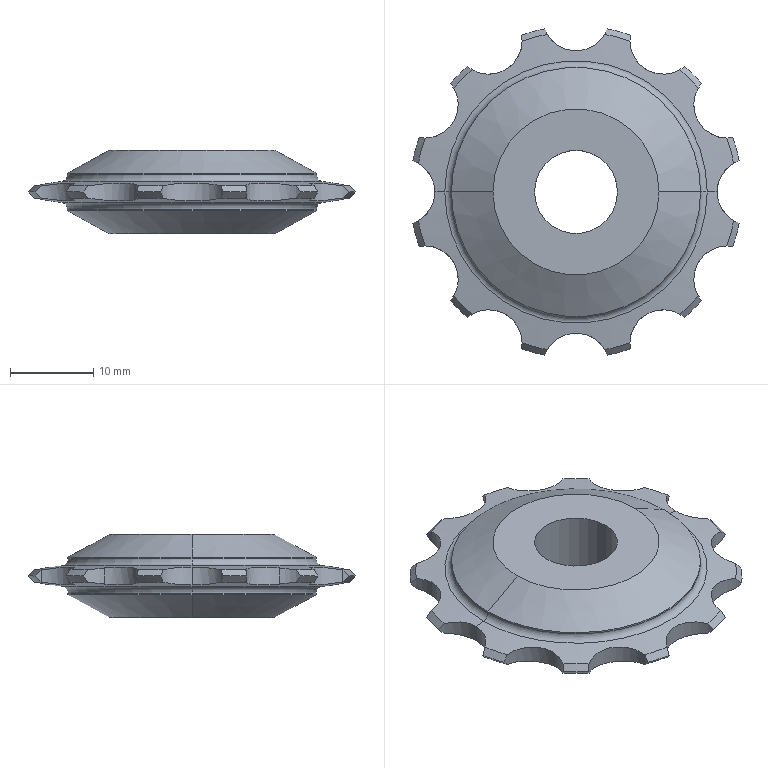Part | STEP file | Deraillieur Wheel | 1 solid | 61 faces | box 39.286 x 39.286 x 10 mm | volume 5894 mm3 | cone 32 | cylinder 23 | torus 4 | plane 2 | commonest cylinder face diameters 8 x17 30 x4 10 x2